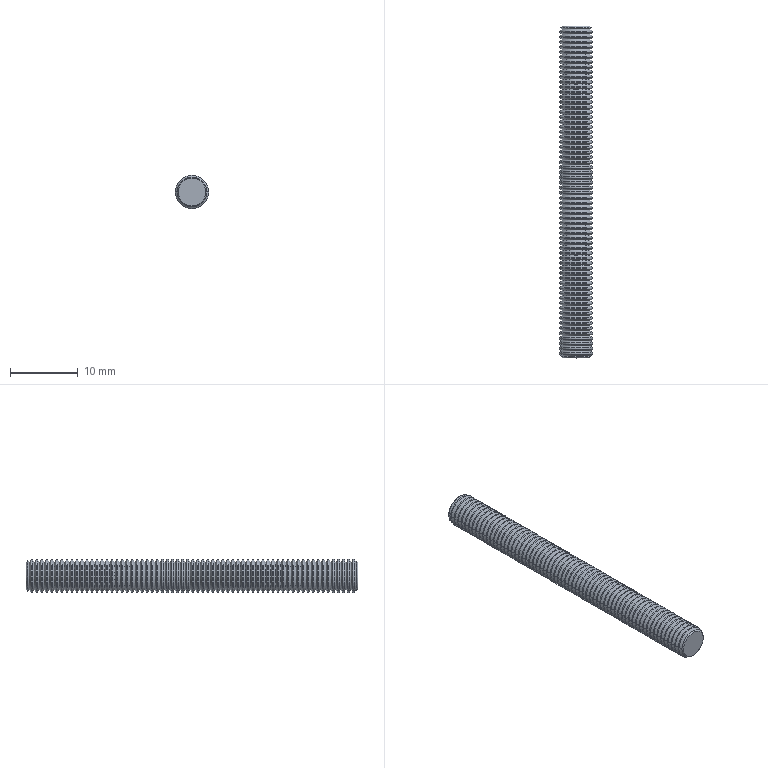Part | STEP file | 1 solid | 400 faces | box 4.9 x 49 x 4.9 mm | volume 811.939 mm3 | cone 268 | cylinder 130 | plane 2 | commonest cylinder face diameters 4.9 x130